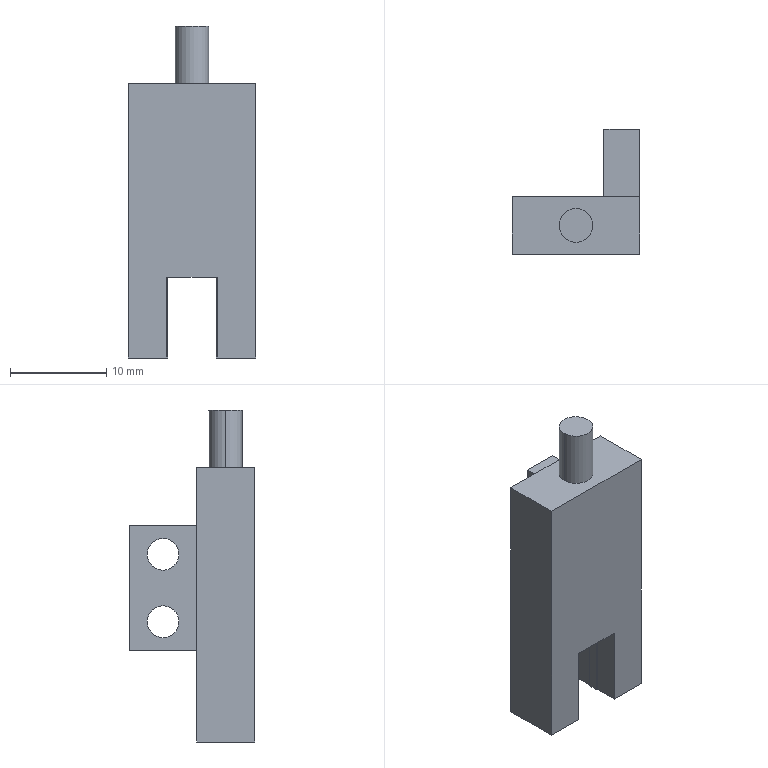Part | STEP file | Slot photoelectric switch FMSM677WR1001 | 2 solids | 30 faces | box 13.2 x 13 x 34.5 mm | volume 2328 mm3 | plane 24 | cylinder 6 | commonest cylinder face diameters 3.3 x4 3.5 x2